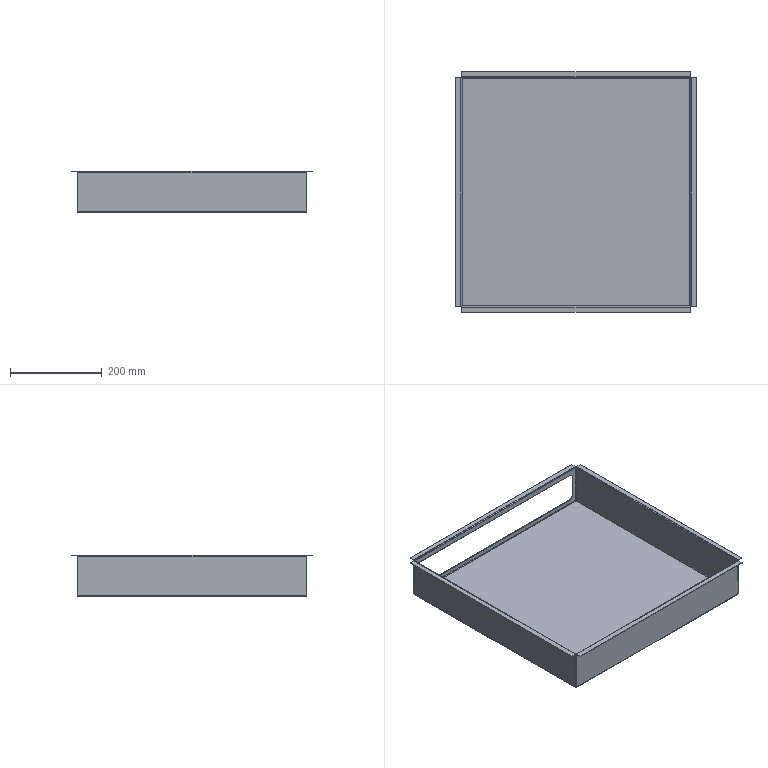Part | SolidWorks | features BaseBody 1 | 1 solid | 102 faces | box 524 x 524 x 91.2 mm | volume 502575 mm3 | plane 82 | cylinder 20 | commonest cylinder face diameters 2 x8 4.4 x8 20 x4